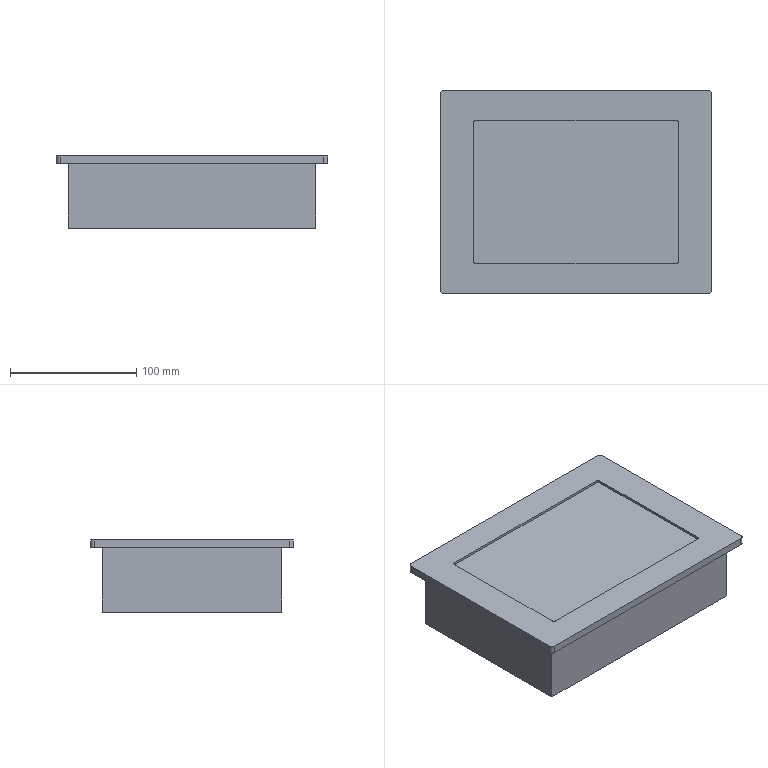Part | SolidWorks | features BaseBody 1 | 1 solid | 24 faces | box 215 x 161 x 57.2 mm | volume 1602281 mm3 | plane 16 | cylinder 8 | commonest cylinder face diameters 4 x4 6 x4
STEP:
#1=CARTESIAN_POINT('',(-81.45,-54.628,-2.));
#2=VERTEX_POINT('',#1);
#3=CARTESIAN_POINT('',(-79.45,-56.628,-2.));
#4=VERTEX_POINT('',#3);
#5=CARTESIAN_POINT('',(-79.45,-54.628,-2.));
#6=DIRECTION('',(0.,0.,1.));
#7=DIRECTION('',(1.,0.,0.));
#8=AXIS2_PLACEMENT_3D('',#5,#6,#7);
#9=CIRCLE('',#8,2.);
#10=EDGE_CURVE('',#2,#4,#9,.T.);
#11=ORIENTED_EDGE('',*,*,#10,.F.);
#12=CARTESIAN_POINT('',(-81.45,-54.628,0.));
#13=VERTEX_POINT('',#12);
#14=CARTESIAN_POINT('',(-81.45,-54.628,-2.));
#15=DIRECTION('',(0.,0.,-1.));
#16=VECTOR('',#15,1000.);
#17=LINE('',#14,#16);
#18=EDGE_CURVE('',#13,#2,#17,.T.);
#19=ORIENTED_EDGE('',*,*,#18,.F.);
#20=CARTESIAN_POINT('',(-79.45,-56.628,0.));
#21=VERTEX_POINT('',#20);
#22=CARTESIAN_POINT('',(-79.45,-54.628,0.));
#23=DIRECTION('',(0.,0.,-1.));
#24=DIRECTION('',(1.,0.,0.));
#25=AXIS2_PLACEMENT_3D('',#22,#23,#24);
#26=CIRCLE('',#25,2.);
#27=EDGE_CURVE('',#21,#13,#26,.T.);
#28=ORIENTED_EDGE('',*,*,#27,.F.);
#29=CARTESIAN_POINT('',(-79.45,-56.628,0.));
#30=DIRECTION('',(0.,0.,1.));
#31=VECTOR('',#30,1000.);
#32=LINE('',#29,#31);
#33=EDGE_CURVE('',#4,#21,#32,.T.);
#34=ORIENTED_EDGE('',*,*,#33,.F.);
#35=EDGE_LOOP('',(#11,#19,#28,#34));
#36=FACE_OUTER_BOUND('',#35,.T.);
#37=CARTESIAN_POINT('',(-79.45,-54.628,-2.));
#38=DIRECTION('',(0.,0.,-1.));
#39=DIRECTION('',(-1.,0.,0.));
#40=AXIS2_PLACEMENT_3D('',#37,#38,#39);
#41=CYLINDRICAL_SURFACE('',#40,2.);
#42=ADVANCED_FACE('',(#36),#41,.F.);
#43=CARTESIAN_POINT('',(-79.45,56.628,-2.));
#44=VERTEX_POINT('',#43);
#45=CARTESIAN_POINT('',(-81.45,54.628,-2.));
#46=VERTEX_POINT('',#45);
#47=CARTESIAN_POINT('',(-79.45,54.628,-2.));
#48=DIRECTION('',(0.,0.,1.));
#49=DIRECTION('',(1.,0.,0.));
#50=AXIS2_PLACEMENT_3D('',#47,#48,#49);
#51=CIRCLE('',#50,2.);
#52=EDGE_CURVE('',#44,#46,#51,.T.);
#53=ORIENTED_EDGE('',*,*,#52,.F.);
#54=CARTESIAN_POINT('',(-79.45,56.628,0.));
#55=VERTEX_POINT('',#54);
#56=CARTESIAN_POINT('',(-79.45,56.628,-2.));
#57=DIRECTION('',(0.,0.,-1.));
#58=VECTOR('',#57,1000.);
#59=LINE('',#56,#58);
#60=EDGE_CURVE('',#55,#44,#59,.T.);
#61=ORIENTED_EDGE('',*,*,#60,.F.);
#62=CARTESIAN_POINT('',(-81.45,54.628,0.));
#63=VERTEX_POINT('',#62);
#64=CARTESIAN_POINT('',(-79.45,54.628,0.));
#65=DIRECTION('',(0.,0.,-1.));
#66=DIRECTION('',(1.,0.,0.));
#67=AXIS2_PLACEMENT_3D('',#64,#65,#66);
#68=CIRCLE('',#67,2.);
#69=EDGE_CURVE('',#63,#55,#68,.T.);
#70=ORIENTED_EDGE('',*,*,#69,.F.);
#71=CARTESIAN_POINT('',(-81.45,54.628,0.));
#72=DIRECTION('',(0.,0.,1.));
#73=VECTOR('',#72,1000.);
#74=LINE('',#71,#73);
#75=EDGE_CURVE('',#46,#63,#74,.T.);
#76=ORIENTED_EDGE('',*,*,#75,.F.);
#77=EDGE_LOOP('',(#53,#61,#70,#76));
#78=FACE_OUTER_BOUND('',#77,.T.);
#79=CARTESIAN_POINT('',(-79.45,54.628,-2.));
#80=DIRECTION('',(0.,0.,-1.));
#81=DIRECTION('',(-1.,0.,0.));
#82=AXIS2_PLACEMENT_3D('',#79,#80,#81);
#83=CYLINDRICAL_SURFACE('',#82,2.);
#84=ADVANCED_FACE('',(#78),#83,.F.);
#85=CARTESIAN_POINT('',(81.45,54.628,-2.));
#86=VERTEX_POINT('',#85);
#87=CARTESIAN_POINT('',(79.45,56.628,-2.));
#88=VERTEX_POINT('',#87);
#89=CARTESIAN_POINT('',(79.45,54.628,-2.));
#90=DIRECTION('',(0.,0.,1.));
#91=DIRECTION('',(1.,0.,0.));
#92=AXIS2_PLACEMENT_3D('',#89,#90,#91);
#93=CIRCLE('',#92,2.);
#94=EDGE_CURVE('',#86,#88,#93,.T.);
#95=ORIENTED_EDGE('',*,*,#94,.F.);
#96=CARTESIAN_POINT('',(81.45,54.628,0.));
#97=VERTEX_POINT('',#96);
#98=CARTESIAN_POINT('',(81.45,54.628,-2.));
#99=DIRECTION('',(0.,0.,-1.));
#100=VECTOR('',#99,1000.);
#101=LINE('',#98,#100);
#102=EDGE_CURVE('',#97,#86,#101,.T.);
#103=ORIENTED_EDGE('',*,*,#102,.F.);
#104=CARTESIAN_POINT('',(79.45,56.628,0.));
#105=VERTEX_POINT('',#104);
#106=CARTESIAN_POINT('',(79.45,54.628,0.));
#107=DIRECTION('',(0.,0.,-1.));
#108=DIRECTION('',(1.,0.,0.));
#109=AXIS2_PLACEMENT_3D('',#106,#107,#108);
#110=CIRCLE('',#109,2.);
#111=EDGE_CURVE('',#105,#97,#110,.T.);
#112=ORIENTED_EDGE('',*,*,#111,.F.);
#113=CARTESIAN_POINT('',(79.45,56.628,0.));
#114=DIRECTION('',(0.,0.,1.));
#115=VECTOR('',#114,1000.);
#116=LINE('',#113,#115);
#117=EDGE_CURVE('',#88,#105,#116,.T.);
#118=ORIENTED_EDGE('',*,*,#117,.F.);
#119=EDGE_LOOP('',(#95,#103,#112,#118));
#120=FACE_OUTER_BOUND('',#119,.T.);
#121=CARTESIAN_POINT('',(79.45,54.628,-2.));
#122=DIRECTION('',(0.,0.,-1.));
#123=DIRECTION('',(-1.,0.,0.));
#124=AXIS2_PLACEMENT_3D('',#121,#122,#123);
#125=CYLINDRICAL_SURFACE('',#124,2.);
#126=ADVANCED_FACE('',(#120),#125,.F.);
#127=CARTESIAN_POINT('',(79.45,-56.628,-2.));
#128=VERTEX_POINT('',#127);
#129=CARTESIAN_POINT('',(81.45,-54.628,-2.));
#130=VERTEX_POINT('',#129);
#131=CARTESIAN_POINT('',(79.45,-54.628,-2.));
#132=DIRECTION('',(0.,0.,1.));
#133=DIRECTION('',(1.,0.,0.));
#134=AXIS2_PLACEMENT_3D('',#131,#132,#133);
#135=CIRCLE('',#134,2.);
#136=EDGE_CURVE('',#128,#130,#135,.T.);
#137=ORIENTED_EDGE('',*,*,#136,.F.);
#138=CARTESIAN_POINT('',(79.45,-56.628,0.));
#139=VERTEX_POINT('',#138);
#140=CARTESIAN_POINT('',(79.45,-56.628,-2.));
#141=DIRECTION('',(0.,0.,-1.));
#142=VECTOR('',#141,1000.);
#143=LINE('',#140,#142);
#144=EDGE_CURVE('',#139,#128,#143,.T.);
#145=ORIENTED_EDGE('',*,*,#144,.F.);
#146=CARTESIAN_POINT('',(81.45,-54.628,0.));
#147=VERTEX_POINT('',#146);
#148=CARTESIAN_POINT('',(79.45,-54.628,0.));
#149=DIRECTION('',(0.,0.,-1.));
#150=DIRECTION('',(1.,0.,0.));
#151=AXIS2_PLACEMENT_3D('',#148,#149,#150);
#152=CIRCLE('',#151,2.);
#153=EDGE_CURVE('',#147,#139,#152,.T.);
#154=ORIENTED_EDGE('',*,*,#153,.F.);
#155=CARTESIAN_POINT('',(81.45,-54.628,0.));
#156=DIRECTION('',(0.,0.,1.));
#157=VECTOR('',#156,1000.);
#158=LINE('',#155,#157);
#159=EDGE_CURVE('',#130,#147,#158,.T.);
#160=ORIENTED_EDGE('',*,*,#159,.F.);
#161=EDGE_LOOP('',(#137,#145,#154,#160));
#162=FACE_OUTER_BOUND('',#161,.T.);
#163=CARTESIAN_POINT('',(79.45,-54.628,-2.));
#164=DIRECTION('',(0.,0.,-1.));
#165=DIRECTION('',(-1.,0.,0.));
#166=AXIS2_PLACEMENT_3D('',#163,#164,#165);
#167=CYLINDRICAL_SURFACE('',#166,2.);
#168=ADVANCED_FACE('',(#162),#167,.F.);
#169=CARTESIAN_POINT('',(104.5,80.5,-6.2));
#170=VERTEX_POINT('',#169);
#171=CARTESIAN_POINT('',(107.5,77.5,-6.2));
#172=VERTEX_POINT('',#171);
#173=CARTESIAN_POINT('',(104.5,77.5,-6.2));
#174=DIRECTION('',(0.,0.,-1.));
#175=DIRECTION('',(1.,0.,0.));
#176=AXIS2_PLACEMENT_3D('',#173,#174,#175);
#177=CIRCLE('',#176,3.);
#178=EDGE_CURVE('',#170,#172,#177,.T.);
#179=ORIENTED_EDGE('',*,*,#178,.F.);
#180=CARTESIAN_POINT('',(104.5,80.5,0.));
#181=VERTEX_POINT('',#180);
#182=CARTESIAN_POINT('',(104.5,80.5,-6.2));
#183=DIRECTION('',(0.,0.,-1.));
#184=VECTOR('',#183,1000.);
#185=LINE('',#182,#184);
#186=EDGE_CURVE('',#181,#170,#185,.T.);
#187=ORIENTED_EDGE('',*,*,#186,.F.);
#188=CARTESIAN_POINT('',(107.5,77.5,0.));
#189=VERTEX_POINT('',#188);
#190=CARTESIAN_POINT('',(104.5,77.5,0.));
#191=DIRECTION('',(0.,0.,1.));
#192=DIRECTION('',(1.,0.,0.));
#193=AXIS2_PLACEMENT_3D('',#190,#191,#192);
#194=CIRCLE('',#193,3.);
#195=EDGE_CURVE('',#189,#181,#194,.T.);
#196=ORIENTED_EDGE('',*,*,#195,.F.);
#197=CARTESIAN_POINT('',(107.5,77.5,-6.2));
#198=DIRECTION('',(0.,0.,1.));
#199=VECTOR('',#198,1000.);
#200=LINE('',#197,#199);
#201=EDGE_CURVE('',#172,#189,#200,.T.);
#202=ORIENTED_EDGE('',*,*,#201,.F.);
#203=EDGE_LOOP('',(#179,#187,#196,#202));
#204=FACE_OUTER_BOUND('',#203,.T.);
#205=CARTESIAN_POINT('',(104.5,77.5,-6.2));
#206=DIRECTION('',(0.,0.,1.));
#207=DIRECTION('',(1.,0.,0.));
#208=AXIS2_PLACEMENT_3D('',#205,#206,#207);
#209=CYLINDRICAL_SURFACE('',#208,3.);
#210=ADVANCED_FACE('',(#204),#209,.T.);
#211=CARTESIAN_POINT('',(107.5,-77.5,-6.2));
#212=VERTEX_POINT('',#211);
#213=CARTESIAN_POINT('',(104.5,-80.5,-6.2));
#214=VERTEX_POINT('',#213);
#215=CARTESIAN_POINT('',(104.5,-77.5,-6.2));
#216=DIRECTION('',(0.,0.,-1.));
#217=DIRECTION('',(1.,0.,0.));
#218=AXIS2_PLACEMENT_3D('',#215,#216,#217);
#219=CIRCLE('',#218,3.);
#220=EDGE_CURVE('',#212,#214,#219,.T.);
#221=ORIENTED_EDGE('',*,*,#220,.F.);
#222=CARTESIAN_POINT('',(107.5,-77.5,0.));
#223=VERTEX_POINT('',#222);
#224=CARTESIAN_POINT('',(107.5,-77.5,-6.2));
#225=DIRECTION('',(0.,0.,-1.));
#226=VECTOR('',#225,1000.);
#227=LINE('',#224,#226);
#228=EDGE_CURVE('',#223,#212,#227,.T.);
#229=ORIENTED_EDGE('',*,*,#228,.F.);
#230=CARTESIAN_POINT('',(104.5,-80.5,0.));
#231=VERTEX_POINT('',#230);
#232=CARTESIAN_POINT('',(104.5,-77.5,0.));
#233=DIRECTION('',(0.,0.,1.));
#234=DIRECTION('',(1.,0.,0.));
#235=AXIS2_PLACEMENT_3D('',#232,#233,#234);
#236=CIRCLE('',#235,3.);
#237=EDGE_CURVE('',#231,#223,#236,.T.);
#238=ORIENTED_EDGE('',*,*,#237,.F.);
#239=CARTESIAN_POINT('',(104.5,-80.5,-6.2));
#240=DIRECTION('',(0.,0.,1.));
#241=VECTOR('',#240,1000.);
#242=LINE('',#239,#241);
#243=EDGE_CURVE('',#214,#231,#242,.T.);
#244=ORIENTED_EDGE('',*,*,#243,.F.);
#245=EDGE_LOOP('',(#221,#229,#238,#244));
#246=FACE_OUTER_BOUND('',#245,.T.);
#247=CARTESIAN_POINT('',(104.5,-77.5,-6.2));
#248=DIRECTION('',(0.,0.,1.));
#249=DIRECTION('',(1.,0.,0.));
#250=AXIS2_PLACEMENT_3D('',#247,#248,#249);
#251=CYLINDRICAL_SURFACE('',#250,3.);
#252=ADVANCED_FACE('',(#246),#251,.T.);
#253=CARTESIAN_POINT('',(-104.5,-80.5,-6.2));
#254=VERTEX_POINT('',#253);
#255=CARTESIAN_POINT('',(-107.5,-77.5,-6.2));
#256=VERTEX_POINT('',#255);
#257=CARTESIAN_POINT('',(-104.5,-77.5,-6.2));
#258=DIRECTION('',(0.,0.,-1.));
#259=DIRECTION('',(1.,0.,0.));
#260=AXIS2_PLACEMENT_3D('',#257,#258,#259);
#261=CIRCLE('',#260,3.);
#262=EDGE_CURVE('',#254,#256,#261,.T.);
#263=ORIENTED_EDGE('',*,*,#262,.F.);
#264=CARTESIAN_POINT('',(-104.5,-80.5,0.));
#265=VERTEX_POINT('',#264);
#266=CARTESIAN_POINT('',(-104.5,-80.5,-6.2));
#267=DIRECTION('',(0.,0.,-1.));
#268=VECTOR('',#267,1000.);
#269=LINE('',#266,#268);
#270=EDGE_CURVE('',#265,#254,#269,.T.);
#271=ORIENTED_EDGE('',*,*,#270,.F.);
#272=CARTESIAN_POINT('',(-107.5,-77.5,0.));
#273=VERTEX_POINT('',#272);
#274=CARTESIAN_POINT('',(-104.5,-77.5,0.));
#275=DIRECTION('',(0.,0.,1.));
#276=DIRECTION('',(1.,0.,0.));
#277=AXIS2_PLACEMENT_3D('',#274,#275,#276);
#278=CIRCLE('',#277,3.);
#279=EDGE_CURVE('',#273,#265,#278,.T.);
#280=ORIENTED_EDGE('',*,*,#279,.F.);
#281=CARTESIAN_POINT('',(-107.5,-77.5,-6.2));
#282=DIRECTION('',(0.,0.,1.));
#283=VECTOR('',#282,1000.);
#284=LINE('',#281,#283);
#285=EDGE_CURVE('',#256,#273,#284,.T.);
#286=ORIENTED_EDGE('',*,*,#285,.F.);
#287=EDGE_LOOP('',(#263,#271,#280,#286));
#288=FACE_OUTER_BOUND('',#287,.T.);
#289=CARTESIAN_POINT('',(-104.5,-77.5,-6.2));
#290=DIRECTION('',(0.,0.,1.));
#291=DIRECTION('',(1.,0.,0.));
#292=AXIS2_PLACEMENT_3D('',#289,#290,#291);
#293=CYLINDRICAL_SURFACE('',#292,3.);
#294=ADVANCED_FACE('',(#288),#293,.T.);
#295=CARTESIAN_POINT('',(-107.5,77.5,-6.2));
#296=VERTEX_POINT('',#295);
#297=CARTESIAN_POINT('',(-104.5,80.5,-6.2));
#298=VERTEX_POINT('',#297);
#299=CARTESIAN_POINT('',(-104.5,77.5,-6.2));
#300=DIRECTION('',(0.,0.,-1.));
#301=DIRECTION('',(1.,0.,0.));
#302=AXIS2_PLACEMENT_3D('',#299,#300,#301);
#303=CIRCLE('',#302,3.);
#304=EDGE_CURVE('',#296,#298,#303,.T.);
#305=ORIENTED_EDGE('',*,*,#304,.F.);
#306=CARTESIAN_POINT('',(-107.5,77.5,0.));
#307=VERTEX_POINT('',#306);
#308=CARTESIAN_POINT('',(-107.5,77.5,-6.2));
#309=DIRECTION('',(0.,0.,-1.));
#310=VECTOR('',#309,1000.);
#311=LINE('',#308,#310);
#312=EDGE_CURVE('',#307,#296,#311,.T.);
#313=ORIENTED_EDGE('',*,*,#312,.F.);
#314=CARTESIAN_POINT('',(-104.5,80.5,0.));
#315=VERTEX_POINT('',#314);
#316=CARTESIAN_POINT('',(-104.5,77.5,0.));
#317=DIRECTION('',(0.,0.,1.));
#318=DIRECTION('',(1.,0.,0.));
#319=AXIS2_PLACEMENT_3D('',#316,#317,#318);
#320=CIRCLE('',#319,3.);
#321=EDGE_CURVE('',#315,#307,#320,.T.);
#322=ORIENTED_EDGE('',*,*,#321,.F.);
#323=CARTESIAN_POINT('',(-104.5,80.5,-6.2));
#324=DIRECTION('',(0.,0.,1.));
#325=VECTOR('',#324,1000.);
#326=LINE('',#323,#325);
#327=EDGE_CURVE('',#298,#315,#326,.T.);
#328=ORIENTED_EDGE('',*,*,#327,.F.);
#329=EDGE_LOOP('',(#305,#313,#322,#328));
#330=FACE_OUTER_BOUND('',#329,.T.);
#331=CARTESIAN_POINT('',(-104.5,77.5,-6.2));
#332=DIRECTION('',(0.,0.,1.));
#333=DIRECTION('',(1.,0.,0.));
#334=AXIS2_PLACEMENT_3D('',#331,#332,#333);
#335=CYLINDRICAL_SURFACE('',#334,3.);
#336=ADVANCED_FACE('',(#330),#335,.T.);
#337=CARTESIAN_POINT('',(-81.45,-56.628,-2.));
#338=DIRECTION('',(1.,0.,0.));
#339=VECTOR('',#338,1000.);
#340=LINE('',#337,#339);
#341=EDGE_CURVE('',#4,#128,#340,.T.);
#342=ORIENTED_EDGE('',*,*,#341,.T.);
#343=ORIENTED_EDGE('',*,*,#136,.T.);
#344=CARTESIAN_POINT('',(81.45,56.628,-2.));
#345=DIRECTION('',(0.,1.,0.));
#346=VECTOR('',#345,1000.);
#347=LINE('',#344,#346);
#348=EDGE_CURVE('',#130,#86,#347,.T.);
#349=ORIENTED_EDGE('',*,*,#348,.T.);
#350=ORIENTED_EDGE('',*,*,#94,.T.);
#351=CARTESIAN_POINT('',(-81.45,56.628,-2.));
#352=DIRECTION('',(-1.,0.,0.));
#353=VECTOR('',#352,1000.);
#354=LINE('',#351,#353);
#355=EDGE_CURVE('',#88,#44,#354,.T.);
#356=ORIENTED_EDGE('',*,*,#355,.T.);
#357=ORIENTED_EDGE('',*,*,#52,.T.);
#358=CARTESIAN_POINT('',(-81.45,56.628,-2.));
#359=DIRECTION('',(0.,-1.,0.));
#360=VECTOR('',#359,1000.);
#361=LINE('',#358,#360);
#362=EDGE_CURVE('',#46,#2,#361,.T.);
#363=ORIENTED_EDGE('',*,*,#362,.T.);
#364=ORIENTED_EDGE('',*,*,#10,.T.);
#365=EDGE_LOOP('',(#342,#343,#349,#350,#356,#357,#363,#364));
#366=FACE_OUTER_BOUND('',#365,.T.);
#367=CARTESIAN_POINT('',(0.,0.,-2.));
#368=DIRECTION('',(0.,0.,1.));
#369=DIRECTION('',(1.,0.,0.));
#370=AXIS2_PLACEMENT_3D('',#367,#368,#369);
#371=PLANE('',#370);
#372=ADVANCED_FACE('',(#366),#371,.T.);
#373=ORIENTED_EDGE('',*,*,#355,.F.);
#374=ORIENTED_EDGE('',*,*,#117,.T.);
#375=CARTESIAN_POINT('',(-81.45,56.628,0.));
#376=DIRECTION('',(-1.,0.,0.));
#377=VECTOR('',#376,1000.);
#378=LINE('',#375,#377);
#379=EDGE_CURVE('',#105,#55,#378,.T.);
#380=ORIENTED_EDGE('',*,*,#379,.T.);
#381=ORIENTED_EDGE('',*,*,#60,.T.);
#382=EDGE_LOOP('',(#373,#374,#380,#381));
#383=FACE_OUTER_BOUND('',#382,.T.);
#384=CARTESIAN_POINT('',(-81.45,56.628,-2.));
#385=DIRECTION('',(0.,1.,0.));
#386=DIRECTION('',(1.,0.,0.));
#387=AXIS2_PLACEMENT_3D('',#384,#385,#386);
#388=PLANE('',#387);
#389=ADVANCED_FACE('',(#383),#388,.F.);
#390=ORIENTED_EDGE('',*,*,#362,.F.);
#391=ORIENTED_EDGE('',*,*,#75,.T.);
#392=CARTESIAN_POINT('',(-81.45,56.628,0.));
#393=DIRECTION('',(0.,-1.,0.));
#394=VECTOR('',#393,1000.);
#395=LINE('',#392,#394);
#396=EDGE_CURVE('',#63,#13,#395,.T.);
#397=ORIENTED_EDGE('',*,*,#396,.T.);
#398=ORIENTED_EDGE('',*,*,#18,.T.);
#399=EDGE_LOOP('',(#390,#391,#397,#398));
#400=FACE_OUTER_BOUND('',#399,.T.);
#401=CARTESIAN_POINT('',(-81.45,56.628,-2.));
#402=DIRECTION('',(-1.,0.,0.));
#403=DIRECTION('',(0.,0.,1.));
#404=AXIS2_PLACEMENT_3D('',#401,#402,#403);
#405=PLANE('',#404);
#406=ADVANCED_FACE('',(#400),#405,.F.);
#407=CARTESIAN_POINT('',(-81.45,-56.628,0.));
#408=DIRECTION('',(1.,0.,0.));
#409=VECTOR('',#408,1000.);
#410=LINE('',#407,#409);
#411=EDGE_CURVE('',#21,#139,#410,.T.);
#412=ORIENTED_EDGE('',*,*,#411,.T.);
#413=ORIENTED_EDGE('',*,*,#144,.T.);
#414=ORIENTED_EDGE('',*,*,#341,.F.);
#415=ORIENTED_EDGE('',*,*,#33,.T.);
#416=EDGE_LOOP('',(#412,#413,#414,#415));
#417=FACE_OUTER_BOUND('',#416,.T.);
#418=CARTESIAN_POINT('',(-81.45,-56.628,-2.));
#419=DIRECTION('',(0.,-1.,0.));
#420=DIRECTION('',(0.,0.,-1.));
#421=AXIS2_PLACEMENT_3D('',#418,#419,#420);
#422=PLANE('',#421);
#423=ADVANCED_FACE('',(#417),#422,.F.);
#424=ORIENTED_EDGE('',*,*,#348,.F.);
#425=ORIENTED_EDGE('',*,*,#159,.T.);
#426=CARTESIAN_POINT('',(81.45,56.628,0.));
#427=DIRECTION('',(0.,1.,0.));
#428=VECTOR('',#427,1000.);
#429=LINE('',#426,#428);
#430=EDGE_CURVE('',#147,#97,#429,.T.);
#431=ORIENTED_EDGE('',*,*,#430,.T.);
#432=ORIENTED_EDGE('',*,*,#102,.T.);
#433=EDGE_LOOP('',(#424,#425,#431,#432));
#434=FACE_OUTER_BOUND('',#433,.T.);
#435=CARTESIAN_POINT('',(81.45,56.628,-2.));
#436=DIRECTION('',(1.,0.,0.));
#437=DIRECTION('',(0.,1.,0.));
#438=AXIS2_PLACEMENT_3D('',#435,#436,#437);
#439=PLANE('',#438);
#440=ADVANCED_FACE('',(#434),#439,.F.);
#441=CARTESIAN_POINT('',(-98.15,-71.15,-57.2));
#442=VERTEX_POINT('',#441);
#443=CARTESIAN_POINT('',(-98.15,71.15,-57.2));
#444=VERTEX_POINT('',#443);
#445=CARTESIAN_POINT('',(-98.15,71.15,-57.2));
#446=DIRECTION('',(0.,1.,0.));
#447=VECTOR('',#446,1000.);
#448=LINE('',#445,#447);
#449=EDGE_CURVE('',#442,#444,#448,.T.);
#450=ORIENTED_EDGE('',*,*,#449,.T.);
#451=CARTESIAN_POINT('',(98.15,71.15,-57.2));
#452=VERTEX_POINT('',#451);
#453=CARTESIAN_POINT('',(98.15,71.15,-57.2));
#454=DIRECTION('',(1.,0.,0.));
#455=VECTOR('',#454,1000.);
#456=LINE('',#453,#455);
#457=EDGE_CURVE('',#444,#452,#456,.T.);
#458=ORIENTED_EDGE('',*,*,#457,.T.);
#459=CARTESIAN_POINT('',(98.15,-71.15,-57.2));
#460=VERTEX_POINT('',#459);
#461=CARTESIAN_POINT('',(98.15,71.15,-57.2));
#462=DIRECTION('',(0.,-1.,0.));
#463=VECTOR('',#462,1000.);
#464=LINE('',#461,#463);
#465=EDGE_CURVE('',#452,#460,#464,.T.);
#466=ORIENTED_EDGE('',*,*,#465,.T.);
#467=CARTESIAN_POINT('',(98.15,-71.15,-57.2));
#468=DIRECTION('',(-1.,0.,0.));
#469=VECTOR('',#468,1000.);
#470=LINE('',#467,#469);
#471=EDGE_CURVE('',#460,#442,#470,.T.);
#472=ORIENTED_EDGE('',*,*,#471,.T.);
#473=EDGE_LOOP('',(#450,#458,#466,#472));
#474=FACE_OUTER_BOUND('',#473,.T.);
#475=CARTESIAN_POINT('',(0.,0.,-57.2));
#476=DIRECTION('',(0.,0.,-1.));
#477=DIRECTION('',(0.,-1.,0.));
#478=AXIS2_PLACEMENT_3D('',#475,#476,#477);
#479=PLANE('',#478);
#480=ADVANCED_FACE('',(#474),#479,.T.);
#481=CARTESIAN_POINT('',(98.15,-71.15,-6.2));
#482=VERTEX_POINT('',#481);
#483=CARTESIAN_POINT('',(-98.15,-71.15,-6.2));
#484=VERTEX_POINT('',#483);
#485=CARTESIAN_POINT('',(98.15,-71.15,-6.2));
#486=DIRECTION('',(-1.,0.,0.));
#487=VECTOR('',#486,1000.);
#488=LINE('',#485,#487);
#489=EDGE_CURVE('',#482,#484,#488,.T.);
#490=ORIENTED_EDGE('',*,*,#489,.T.);
#491=CARTESIAN_POINT('',(-98.15,-71.15,-57.2));
#492=DIRECTION('',(0.,0.,1.));
#493=VECTOR('',#492,1000.);
#494=LINE('',#491,#493);
#495=EDGE_CURVE('',#442,#484,#494,.T.);
#496=ORIENTED_EDGE('',*,*,#495,.F.);
#497=ORIENTED_EDGE('',*,*,#471,.F.);
#498=CARTESIAN_POINT('',(98.15,-71.15,-57.2));
#499=DIRECTION('',(0.,0.,1.));
#500=VECTOR('',#499,1000.);
#501=LINE('',#498,#500);
#502=EDGE_CURVE('',#460,#482,#501,.T.);
#503=ORIENTED_EDGE('',*,*,#502,.T.);
#504=EDGE_LOOP('',(#490,#496,#497,#503));
#505=FACE_OUTER_BOUND('',#504,.T.);
#506=CARTESIAN_POINT('',(98.15,-71.15,-57.2));
#507=DIRECTION('',(0.,1.,0.));
#508=DIRECTION('',(1.,0.,0.));
#509=AXIS2_PLACEMENT_3D('',#506,#507,#508);
#510=PLANE('',#509);
#511=ADVANCED_FACE('',(#505),#510,.F.);
#512=CARTESIAN_POINT('',(98.15,71.15,-6.2));
#513=VERTEX_POINT('',#512);
#514=CARTESIAN_POINT('',(98.15,71.15,-6.2));
#515=DIRECTION('',(0.,-1.,0.));
#516=VECTOR('',#515,1000.);
#517=LINE('',#514,#516);
#518=EDGE_CURVE('',#513,#482,#517,.T.);
#519=ORIENTED_EDGE('',*,*,#518,.T.);
#520=ORIENTED_EDGE('',*,*,#502,.F.);
#521=ORIENTED_EDGE('',*,*,#465,.F.);
#522=CARTESIAN_POINT('',(98.15,71.15,-57.2));
#523=DIRECTION('',(0.,0.,1.));
#524=VECTOR('',#523,1000.);
#525=LINE('',#522,#524);
#526=EDGE_CURVE('',#452,#513,#525,.T.);
#527=ORIENTED_EDGE('',*,*,#526,.T.);
#528=EDGE_LOOP('',(#519,#520,#521,#527));
#529=FACE_OUTER_BOUND('',#528,.T.);
#530=CARTESIAN_POINT('',(98.15,71.15,-57.2));
#531=DIRECTION('',(-1.,0.,0.));
#532=DIRECTION('',(0.,0.,1.));
#533=AXIS2_PLACEMENT_3D('',#530,#531,#532);
#534=PLANE('',#533);
#535=ADVANCED_FACE('',(#529),#534,.F.);
#536=CARTESIAN_POINT('',(-98.15,71.15,-6.2));
#537=VERTEX_POINT('',#536);
#538=CARTESIAN_POINT('',(98.15,71.15,-6.2));
#539=DIRECTION('',(1.,0.,0.));
#540=VECTOR('',#539,1000.);
#541=LINE('',#538,#540);
#542=EDGE_CURVE('',#537,#513,#541,.T.);
#543=ORIENTED_EDGE('',*,*,#542,.T.);
#544=ORIENTED_EDGE('',*,*,#526,.F.);
#545=ORIENTED_EDGE('',*,*,#457,.F.);
#546=CARTESIAN_POINT('',(-98.15,71.15,-57.2));
#547=DIRECTION('',(0.,0.,1.));
#548=VECTOR('',#547,1000.);
#549=LINE('',#546,#548);
#550=EDGE_CURVE('',#444,#537,#549,.T.);
#551=ORIENTED_EDGE('',*,*,#550,.T.);
#552=EDGE_LOOP('',(#543,#544,#545,#551));
#553=FACE_OUTER_BOUND('',#552,.T.);
#554=CARTESIAN_POINT('',(98.15,71.15,-57.2));
#555=DIRECTION('',(0.,-1.,0.));
#556=DIRECTION('',(0.,0.,-1.));
#557=AXIS2_PLACEMENT_3D('',#554,#555,#556);
#558=PLANE('',#557);
#559=ADVANCED_FACE('',(#553),#558,.F.);
#560=CARTESIAN_POINT('',(-98.15,71.15,-6.2));
#561=DIRECTION('',(0.,1.,0.));
#562=VECTOR('',#561,1000.);
#563=LINE('',#560,#562);
#564=EDGE_CURVE('',#484,#537,#563,.T.);
#565=ORIENTED_EDGE('',*,*,#564,.T.);
#566=ORIENTED_EDGE('',*,*,#550,.F.);
#567=ORIENTED_EDGE('',*,*,#449,.F.);
#568=ORIENTED_EDGE('',*,*,#495,.T.);
#569=EDGE_LOOP('',(#565,#566,#567,#568));
#570=FACE_OUTER_BOUND('',#569,.T.);
#571=CARTESIAN_POINT('',(-98.15,71.15,-57.2));
#572=DIRECTION('',(1.,0.,0.));
#573=DIRECTION('',(0.,-1.,0.));
#574=AXIS2_PLACEMENT_3D('',#571,#572,#573);
#575=PLANE('',#574);
#576=ADVANCED_FACE('',(#570),#575,.F.);
#577=ORIENTED_EDGE('',*,*,#430,.F.);
#578=ORIENTED_EDGE('',*,*,#153,.T.);
#579=ORIENTED_EDGE('',*,*,#411,.F.);
#580=ORIENTED_EDGE('',*,*,#27,.T.);
#581=ORIENTED_EDGE('',*,*,#396,.F.);
#582=ORIENTED_EDGE('',*,*,#69,.T.);
#583=ORIENTED_EDGE('',*,*,#379,.F.);
#584=ORIENTED_EDGE('',*,*,#111,.T.);
#585=EDGE_LOOP('',(#577,#578,#579,#580,#581,#582,#583,#584));
#586=FACE_BOUND('',#585,.T.);
#587=CARTESIAN_POINT('',(-107.5,80.5,0.));
#588=DIRECTION('',(-1.,0.,0.));
#589=VECTOR('',#588,1000.);
#590=LINE('',#587,#589);
#591=EDGE_CURVE('',#181,#315,#590,.T.);
#592=ORIENTED_EDGE('',*,*,#591,.T.);
#593=ORIENTED_EDGE('',*,*,#321,.T.);
#594=CARTESIAN_POINT('',(-107.5,80.5,0.));
#595=DIRECTION('',(0.,-1.,0.));
#596=VECTOR('',#595,1000.);
#597=LINE('',#594,#596);
#598=EDGE_CURVE('',#307,#273,#597,.T.);
#599=ORIENTED_EDGE('',*,*,#598,.T.);
#600=ORIENTED_EDGE('',*,*,#279,.T.);
#601=CARTESIAN_POINT('',(-107.5,-80.5,0.));
#602=DIRECTION('',(1.,0.,0.));
#603=VECTOR('',#602,1000.);
#604=LINE('',#601,#603);
#605=EDGE_CURVE('',#265,#231,#604,.T.);
#606=ORIENTED_EDGE('',*,*,#605,.T.);
#607=ORIENTED_EDGE('',*,*,#237,.T.);
#608=CARTESIAN_POINT('',(107.5,80.5,0.));
#609=DIRECTION('',(0.,1.,0.));
#610=VECTOR('',#609,1000.);
#611=LINE('',#608,#610);
#612=EDGE_CURVE('',#223,#189,#611,.T.);
#613=ORIENTED_EDGE('',*,*,#612,.T.);
#614=ORIENTED_EDGE('',*,*,#195,.T.);
#615=EDGE_LOOP('',(#592,#593,#599,#600,#606,#607,#613,#614));
#616=FACE_OUTER_BOUND('',#615,.T.);
#617=CARTESIAN_POINT('',(0.,0.,0.));
#618=DIRECTION('',(0.,0.,1.));
#619=DIRECTION('',(1.,0.,0.));
#620=AXIS2_PLACEMENT_3D('',#617,#618,#619);
#621=PLANE('',#620);
#622=ADVANCED_FACE('',(#586,#616),#621,.T.);
#623=CARTESIAN_POINT('',(-107.5,80.5,-6.2));
#624=DIRECTION('',(-1.,0.,0.));
#625=VECTOR('',#624,1000.);
#626=LINE('',#623,#625);
#627=EDGE_CURVE('',#170,#298,#626,.T.);
#628=ORIENTED_EDGE('',*,*,#627,.T.);
#629=ORIENTED_EDGE('',*,*,#327,.T.);
#630=ORIENTED_EDGE('',*,*,#591,.F.);
#631=ORIENTED_EDGE('',*,*,#186,.T.);
#632=EDGE_LOOP('',(#628,#629,#630,#631));
#633=FACE_OUTER_BOUND('',#632,.T.);
#634=CARTESIAN_POINT('',(-107.5,80.5,-6.2));
#635=DIRECTION('',(0.,1.,0.));
#636=DIRECTION('',(1.,0.,0.));
#637=AXIS2_PLACEMENT_3D('',#634,#635,#636);
#638=PLANE('',#637);
#639=ADVANCED_FACE('',(#633),#638,.T.);
#640=ORIENTED_EDGE('',*,*,#598,.F.);
#641=ORIENTED_EDGE('',*,*,#312,.T.);
#642=CARTESIAN_POINT('',(-107.5,80.5,-6.2));
#643=DIRECTION('',(0.,-1.,0.));
#644=VECTOR('',#643,1000.);
#645=LINE('',#642,#644);
#646=EDGE_CURVE('',#296,#256,#645,.T.);
#647=ORIENTED_EDGE('',*,*,#646,.T.);
#648=ORIENTED_EDGE('',*,*,#285,.T.);
#649=EDGE_LOOP('',(#640,#641,#647,#648));
#650=FACE_OUTER_BOUND('',#649,.T.);
#651=CARTESIAN_POINT('',(-107.5,80.5,-6.2));
#652=DIRECTION('',(-1.,0.,0.));
#653=DIRECTION('',(0.,1.,0.));
#654=AXIS2_PLACEMENT_3D('',#651,#652,#653);
#655=PLANE('',#654);
#656=ADVANCED_FACE('',(#650),#655,.T.);
#657=ORIENTED_EDGE('',*,*,#605,.F.);
#658=ORIENTED_EDGE('',*,*,#270,.T.);
#659=CARTESIAN_POINT('',(-107.5,-80.5,-6.2));
#660=DIRECTION('',(1.,0.,0.));
#661=VECTOR('',#660,1000.);
#662=LINE('',#659,#661);
#663=EDGE_CURVE('',#254,#214,#662,.T.);
#664=ORIENTED_EDGE('',*,*,#663,.T.);
#665=ORIENTED_EDGE('',*,*,#243,.T.);
#666=EDGE_LOOP('',(#657,#658,#664,#665));
#667=FACE_OUTER_BOUND('',#666,.T.);
#668=CARTESIAN_POINT('',(-107.5,-80.5,-6.2));
#669=DIRECTION('',(0.,-1.,0.));
#670=DIRECTION('',(0.,0.,-1.));
#671=AXIS2_PLACEMENT_3D('',#668,#669,#670);
#672=PLANE('',#671);
#673=ADVANCED_FACE('',(#667),#672,.T.);
#674=ORIENTED_EDGE('',*,*,#612,.F.);
#675=ORIENTED_EDGE('',*,*,#228,.T.);
#676=CARTESIAN_POINT('',(107.5,80.5,-6.2));
#677=DIRECTION('',(0.,1.,0.));
#678=VECTOR('',#677,1000.);
#679=LINE('',#676,#678);
#680=EDGE_CURVE('',#212,#172,#679,.T.);
#681=ORIENTED_EDGE('',*,*,#680,.T.);
#682=ORIENTED_EDGE('',*,*,#201,.T.);
#683=EDGE_LOOP('',(#674,#675,#681,#682));
#684=FACE_OUTER_BOUND('',#683,.T.);
#685=CARTESIAN_POINT('',(107.5,80.5,-6.2));
#686=DIRECTION('',(1.,0.,0.));
#687=DIRECTION('',(0.,1.,0.));
#688=AXIS2_PLACEMENT_3D('',#685,#686,#687);
#689=PLANE('',#688);
#690=ADVANCED_FACE('',(#684),#689,.T.);
#691=ORIENTED_EDGE('',*,*,#564,.F.);
#692=ORIENTED_EDGE('',*,*,#489,.F.);
#693=ORIENTED_EDGE('',*,*,#518,.F.);
#694=ORIENTED_EDGE('',*,*,#542,.F.);
#695=EDGE_LOOP('',(#691,#692,#693,#694));
#696=FACE_BOUND('',#695,.T.);
#697=ORIENTED_EDGE('',*,*,#646,.F.);
#698=ORIENTED_EDGE('',*,*,#304,.T.);
#699=ORIENTED_EDGE('',*,*,#627,.F.);
#700=ORIENTED_EDGE('',*,*,#178,.T.);
#701=ORIENTED_EDGE('',*,*,#680,.F.);
#702=ORIENTED_EDGE('',*,*,#220,.T.);
#703=ORIENTED_EDGE('',*,*,#663,.F.);
#704=ORIENTED_EDGE('',*,*,#262,.T.);
#705=EDGE_LOOP('',(#697,#698,#699,#700,#701,#702,#703,#704));
#706=FACE_OUTER_BOUND('',#705,.T.);
#707=CARTESIAN_POINT('',(0.,0.,-6.2));
#708=DIRECTION('',(0.,0.,1.));
#709=DIRECTION('',(1.,0.,0.));
#710=AXIS2_PLACEMENT_3D('',#707,#708,#709);
#711=PLANE('',#710);
#712=ADVANCED_FACE('',(#696,#706),#711,.F.);
#713=CLOSED_SHELL('',(#42,#84,#126,#168,#210,#252,#294,#336,#372,#389,#406,#423,#440,#480,#511,#535,#559,#576,#622,#639,#656,#673,#690,#712));
#714=MANIFOLD_SOLID_BREP('',#713);
#715=CARTESIAN_POINT('',(0.,0.,0.));
#716=DIRECTION('',(0.,0.,1.));
#717=DIRECTION('',(1.,0.,0.));
#718=AXIS2_PLACEMENT_3D('',#715,#716,#717);
#719=(LENGTH_UNIT()NAMED_UNIT(*)SI_UNIT(.MILLI.,.METRE.));
#720=UNCERTAINTY_MEASURE_WITH_UNIT(LENGTH_MEASURE(0.00001),#719,'','');
#721=(NAMED_UNIT(*)PLANE_ANGLE_UNIT()SI_UNIT($,.RADIAN.));
#722=(NAMED_UNIT(*)SI_UNIT($,.STERADIAN.)SOLID_ANGLE_UNIT());
#723=(GEOMETRIC_REPRESENTATION_CONTEXT(3)GLOBAL_UNCERTAINTY_ASSIGNED_CONTEXT((#720))GLOBAL_UNIT_ASSIGNED_CONTEXT((#719,#721,#722))REPRESENTATION_CONTEXT('',''));
#724=ADVANCED_BREP_SHAPE_REPRESENTATION('',(#714,#718),#723);